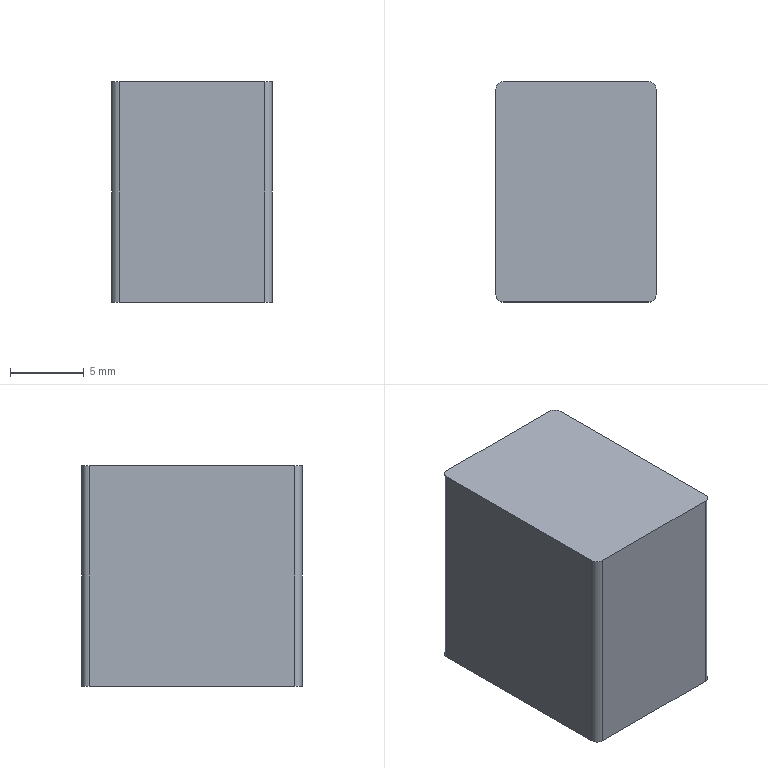Part | NX | features BREP 1 | 1 solid | 10 faces | box 10.887 x 14.955 x 15 mm | volume 2439 mm3 | plane 6 | cylinder 4 | commonest cylinder face diameters 1 x4
STEP:
#1=CARTESIAN_POINT('',(-4.944,7.478,-25.6));
#2=VERTEX_POINT('',#1);
#3=CARTESIAN_POINT('',(-5.444,6.978,-25.6));
#4=VERTEX_POINT('',#3);
#5=CARTESIAN_POINT('',(-4.944,6.978,-25.6));
#6=DIRECTION('',(0.,0.,1.));
#7=DIRECTION('',(1.,0.,0.));
#8=AXIS2_PLACEMENT_3D('',#5,#6,#7);
#9=CIRCLE('',#8,0.5);
#10=EDGE_CURVE('',#2,#4,#9,.T.);
#11=ORIENTED_EDGE('',*,*,#10,.F.);
#12=CARTESIAN_POINT('',(-4.944,7.478,-40.6));
#13=VERTEX_POINT('',#12);
#14=CARTESIAN_POINT('',(-4.944,7.478,-40.6));
#15=DIRECTION('',(0.,0.,1.));
#16=VECTOR('',#15,1000.);
#17=LINE('',#14,#16);
#18=EDGE_CURVE('',#13,#2,#17,.T.);
#19=ORIENTED_EDGE('',*,*,#18,.F.);
#20=CARTESIAN_POINT('',(-5.444,6.978,-40.6));
#21=VERTEX_POINT('',#20);
#22=CARTESIAN_POINT('',(-4.944,6.978,-40.6));
#23=DIRECTION('',(0.,0.,1.));
#24=DIRECTION('',(1.,0.,0.));
#25=AXIS2_PLACEMENT_3D('',#22,#23,#24);
#26=CIRCLE('',#25,0.5);
#27=EDGE_CURVE('',#13,#21,#26,.T.);
#28=ORIENTED_EDGE('',*,*,#27,.T.);
#29=CARTESIAN_POINT('',(-5.444,6.978,-40.6));
#30=DIRECTION('',(0.,0.,1.));
#31=VECTOR('',#30,1000.);
#32=LINE('',#29,#31);
#33=EDGE_CURVE('',#21,#4,#32,.T.);
#34=ORIENTED_EDGE('',*,*,#33,.T.);
#35=EDGE_LOOP('',(#11,#19,#28,#34));
#36=FACE_BOUND('',#35,.T.);
#37=CARTESIAN_POINT('',(-4.944,6.978,-40.6));
#38=DIRECTION('',(0.,0.,1.));
#39=DIRECTION('',(-1.,0.,0.));
#40=AXIS2_PLACEMENT_3D('',#37,#38,#39);
#41=CYLINDRICAL_SURFACE('',#40,0.5);
#42=ADVANCED_FACE('',(#36),#41,.T.);
#43=CARTESIAN_POINT('',(-5.444,-6.978,-25.6));
#44=VERTEX_POINT('',#43);
#45=CARTESIAN_POINT('',(-5.444,-6.978,-25.6));
#46=DIRECTION('',(0.,1.,0.));
#47=VECTOR('',#46,1000.);
#48=LINE('',#45,#47);
#49=EDGE_CURVE('',#44,#4,#48,.T.);
#50=ORIENTED_EDGE('',*,*,#49,.T.);
#51=ORIENTED_EDGE('',*,*,#33,.F.);
#52=CARTESIAN_POINT('',(-5.444,-6.978,-40.6));
#53=VERTEX_POINT('',#52);
#54=CARTESIAN_POINT('',(-5.444,-6.978,-40.6));
#55=DIRECTION('',(0.,1.,0.));
#56=VECTOR('',#55,1000.);
#57=LINE('',#54,#56);
#58=EDGE_CURVE('',#53,#21,#57,.T.);
#59=ORIENTED_EDGE('',*,*,#58,.F.);
#60=CARTESIAN_POINT('',(-5.444,-6.978,-40.6));
#61=DIRECTION('',(0.,0.,1.));
#62=VECTOR('',#61,1000.);
#63=LINE('',#60,#62);
#64=EDGE_CURVE('',#53,#44,#63,.T.);
#65=ORIENTED_EDGE('',*,*,#64,.T.);
#66=EDGE_LOOP('',(#50,#51,#59,#65));
#67=FACE_BOUND('',#66,.T.);
#68=CARTESIAN_POINT('',(-5.444,-6.978,-40.6));
#69=DIRECTION('',(1.,0.,0.));
#70=DIRECTION('',(0.,-1.,0.));
#71=AXIS2_PLACEMENT_3D('',#68,#69,#70);
#72=PLANE('',#71);
#73=ADVANCED_FACE('',(#67),#72,.F.);
#74=CARTESIAN_POINT('',(-4.944,-7.478,-25.6));
#75=VERTEX_POINT('',#74);
#76=CARTESIAN_POINT('',(-4.944,-6.978,-25.6));
#77=DIRECTION('',(0.,0.,1.));
#78=DIRECTION('',(1.,0.,0.));
#79=AXIS2_PLACEMENT_3D('',#76,#77,#78);
#80=CIRCLE('',#79,0.5);
#81=EDGE_CURVE('',#44,#75,#80,.T.);
#82=ORIENTED_EDGE('',*,*,#81,.F.);
#83=ORIENTED_EDGE('',*,*,#64,.F.);
#84=CARTESIAN_POINT('',(-4.944,-7.478,-40.6));
#85=VERTEX_POINT('',#84);
#86=CARTESIAN_POINT('',(-4.944,-6.978,-40.6));
#87=DIRECTION('',(0.,0.,1.));
#88=DIRECTION('',(1.,0.,0.));
#89=AXIS2_PLACEMENT_3D('',#86,#87,#88);
#90=CIRCLE('',#89,0.5);
#91=EDGE_CURVE('',#53,#85,#90,.T.);
#92=ORIENTED_EDGE('',*,*,#91,.T.);
#93=CARTESIAN_POINT('',(-4.944,-7.478,-40.6));
#94=DIRECTION('',(0.,0.,1.));
#95=VECTOR('',#94,1000.);
#96=LINE('',#93,#95);
#97=EDGE_CURVE('',#85,#75,#96,.T.);
#98=ORIENTED_EDGE('',*,*,#97,.T.);
#99=EDGE_LOOP('',(#82,#83,#92,#98));
#100=FACE_BOUND('',#99,.T.);
#101=CARTESIAN_POINT('',(-4.944,-6.978,-40.6));
#102=DIRECTION('',(0.,0.,1.));
#103=DIRECTION('',(-1.,0.,0.));
#104=AXIS2_PLACEMENT_3D('',#101,#102,#103);
#105=CYLINDRICAL_SURFACE('',#104,0.5);
#106=ADVANCED_FACE('',(#100),#105,.T.);
#107=CARTESIAN_POINT('',(4.944,-7.478,-25.6));
#108=VERTEX_POINT('',#107);
#109=CARTESIAN_POINT('',(4.944,-7.478,-25.6));
#110=DIRECTION('',(-1.,0.,0.));
#111=VECTOR('',#110,1000.);
#112=LINE('',#109,#111);
#113=EDGE_CURVE('',#108,#75,#112,.T.);
#114=ORIENTED_EDGE('',*,*,#113,.T.);
#115=ORIENTED_EDGE('',*,*,#97,.F.);
#116=CARTESIAN_POINT('',(4.944,-7.478,-40.6));
#117=VERTEX_POINT('',#116);
#118=CARTESIAN_POINT('',(4.944,-7.478,-40.6));
#119=DIRECTION('',(-1.,0.,0.));
#120=VECTOR('',#119,1000.);
#121=LINE('',#118,#120);
#122=EDGE_CURVE('',#117,#85,#121,.T.);
#123=ORIENTED_EDGE('',*,*,#122,.F.);
#124=CARTESIAN_POINT('',(4.944,-7.478,-40.6));
#125=DIRECTION('',(0.,0.,1.));
#126=VECTOR('',#125,1000.);
#127=LINE('',#124,#126);
#128=EDGE_CURVE('',#117,#108,#127,.T.);
#129=ORIENTED_EDGE('',*,*,#128,.T.);
#130=EDGE_LOOP('',(#114,#115,#123,#129));
#131=FACE_BOUND('',#130,.T.);
#132=CARTESIAN_POINT('',(4.944,-7.478,-40.6));
#133=DIRECTION('',(0.,1.,0.));
#134=DIRECTION('',(1.,0.,0.));
#135=AXIS2_PLACEMENT_3D('',#132,#133,#134);
#136=PLANE('',#135);
#137=ADVANCED_FACE('',(#131),#136,.F.);
#138=CARTESIAN_POINT('',(5.444,-6.978,-25.6));
#139=VERTEX_POINT('',#138);
#140=CARTESIAN_POINT('',(4.944,-6.978,-25.6));
#141=DIRECTION('',(0.,0.,1.));
#142=DIRECTION('',(1.,0.,0.));
#143=AXIS2_PLACEMENT_3D('',#140,#141,#142);
#144=CIRCLE('',#143,0.5);
#145=EDGE_CURVE('',#108,#139,#144,.T.);
#146=ORIENTED_EDGE('',*,*,#145,.F.);
#147=ORIENTED_EDGE('',*,*,#128,.F.);
#148=CARTESIAN_POINT('',(5.444,-6.978,-40.6));
#149=VERTEX_POINT('',#148);
#150=CARTESIAN_POINT('',(4.944,-6.978,-40.6));
#151=DIRECTION('',(0.,0.,1.));
#152=DIRECTION('',(1.,0.,0.));
#153=AXIS2_PLACEMENT_3D('',#150,#151,#152);
#154=CIRCLE('',#153,0.5);
#155=EDGE_CURVE('',#117,#149,#154,.T.);
#156=ORIENTED_EDGE('',*,*,#155,.T.);
#157=CARTESIAN_POINT('',(5.444,-6.978,-40.6));
#158=DIRECTION('',(0.,0.,1.));
#159=VECTOR('',#158,1000.);
#160=LINE('',#157,#159);
#161=EDGE_CURVE('',#149,#139,#160,.T.);
#162=ORIENTED_EDGE('',*,*,#161,.T.);
#163=EDGE_LOOP('',(#146,#147,#156,#162));
#164=FACE_BOUND('',#163,.T.);
#165=CARTESIAN_POINT('',(4.944,-6.978,-40.6));
#166=DIRECTION('',(0.,0.,1.));
#167=DIRECTION('',(-1.,0.,0.));
#168=AXIS2_PLACEMENT_3D('',#165,#166,#167);
#169=CYLINDRICAL_SURFACE('',#168,0.5);
#170=ADVANCED_FACE('',(#164),#169,.T.);
#171=CARTESIAN_POINT('',(5.444,6.978,-25.6));
#172=VERTEX_POINT('',#171);
#173=CARTESIAN_POINT('',(5.444,6.978,-25.6));
#174=DIRECTION('',(0.,-1.,0.));
#175=VECTOR('',#174,1000.);
#176=LINE('',#173,#175);
#177=EDGE_CURVE('',#172,#139,#176,.T.);
#178=ORIENTED_EDGE('',*,*,#177,.T.);
#179=ORIENTED_EDGE('',*,*,#161,.F.);
#180=CARTESIAN_POINT('',(5.444,6.978,-40.6));
#181=VERTEX_POINT('',#180);
#182=CARTESIAN_POINT('',(5.444,6.978,-40.6));
#183=DIRECTION('',(0.,-1.,0.));
#184=VECTOR('',#183,1000.);
#185=LINE('',#182,#184);
#186=EDGE_CURVE('',#181,#149,#185,.T.);
#187=ORIENTED_EDGE('',*,*,#186,.F.);
#188=CARTESIAN_POINT('',(5.444,6.978,-40.6));
#189=DIRECTION('',(0.,0.,1.));
#190=VECTOR('',#189,1000.);
#191=LINE('',#188,#190);
#192=EDGE_CURVE('',#181,#172,#191,.T.);
#193=ORIENTED_EDGE('',*,*,#192,.T.);
#194=EDGE_LOOP('',(#178,#179,#187,#193));
#195=FACE_BOUND('',#194,.T.);
#196=CARTESIAN_POINT('',(5.444,6.978,-40.6));
#197=DIRECTION('',(-1.,0.,0.));
#198=DIRECTION('',(0.,0.,-1.));
#199=AXIS2_PLACEMENT_3D('',#196,#197,#198);
#200=PLANE('',#199);
#201=ADVANCED_FACE('',(#195),#200,.F.);
#202=CARTESIAN_POINT('',(4.944,7.478,-25.6));
#203=VERTEX_POINT('',#202);
#204=CARTESIAN_POINT('',(4.944,6.978,-25.6));
#205=DIRECTION('',(0.,0.,1.));
#206=DIRECTION('',(1.,0.,0.));
#207=AXIS2_PLACEMENT_3D('',#204,#205,#206);
#208=CIRCLE('',#207,0.5);
#209=EDGE_CURVE('',#172,#203,#208,.T.);
#210=ORIENTED_EDGE('',*,*,#209,.F.);
#211=ORIENTED_EDGE('',*,*,#192,.F.);
#212=CARTESIAN_POINT('',(4.944,7.478,-40.6));
#213=VERTEX_POINT('',#212);
#214=CARTESIAN_POINT('',(4.944,6.978,-40.6));
#215=DIRECTION('',(0.,0.,1.));
#216=DIRECTION('',(1.,0.,0.));
#217=AXIS2_PLACEMENT_3D('',#214,#215,#216);
#218=CIRCLE('',#217,0.5);
#219=EDGE_CURVE('',#181,#213,#218,.T.);
#220=ORIENTED_EDGE('',*,*,#219,.T.);
#221=CARTESIAN_POINT('',(4.944,7.478,-40.6));
#222=DIRECTION('',(0.,0.,1.));
#223=VECTOR('',#222,1000.);
#224=LINE('',#221,#223);
#225=EDGE_CURVE('',#213,#203,#224,.T.);
#226=ORIENTED_EDGE('',*,*,#225,.T.);
#227=EDGE_LOOP('',(#210,#211,#220,#226));
#228=FACE_BOUND('',#227,.T.);
#229=CARTESIAN_POINT('',(4.944,6.978,-40.6));
#230=DIRECTION('',(0.,0.,1.));
#231=DIRECTION('',(-1.,0.,0.));
#232=AXIS2_PLACEMENT_3D('',#229,#230,#231);
#233=CYLINDRICAL_SURFACE('',#232,0.5);
#234=ADVANCED_FACE('',(#228),#233,.T.);
#235=CARTESIAN_POINT('',(-4.944,7.478,-25.6));
#236=DIRECTION('',(1.,0.,0.));
#237=VECTOR('',#236,1000.);
#238=LINE('',#235,#237);
#239=EDGE_CURVE('',#2,#203,#238,.T.);
#240=ORIENTED_EDGE('',*,*,#239,.T.);
#241=ORIENTED_EDGE('',*,*,#225,.F.);
#242=CARTESIAN_POINT('',(-4.944,7.478,-40.6));
#243=DIRECTION('',(1.,0.,0.));
#244=VECTOR('',#243,1000.);
#245=LINE('',#242,#244);
#246=EDGE_CURVE('',#13,#213,#245,.T.);
#247=ORIENTED_EDGE('',*,*,#246,.F.);
#248=ORIENTED_EDGE('',*,*,#18,.T.);
#249=EDGE_LOOP('',(#240,#241,#247,#248));
#250=FACE_BOUND('',#249,.T.);
#251=CARTESIAN_POINT('',(-4.944,7.478,-40.6));
#252=DIRECTION('',(0.,-1.,0.));
#253=DIRECTION('',(0.,0.,1.));
#254=AXIS2_PLACEMENT_3D('',#251,#252,#253);
#255=PLANE('',#254);
#256=ADVANCED_FACE('',(#250),#255,.F.);
#257=ORIENTED_EDGE('',*,*,#27,.F.);
#258=ORIENTED_EDGE('',*,*,#246,.T.);
#259=ORIENTED_EDGE('',*,*,#219,.F.);
#260=ORIENTED_EDGE('',*,*,#186,.T.);
#261=ORIENTED_EDGE('',*,*,#155,.F.);
#262=ORIENTED_EDGE('',*,*,#122,.T.);
#263=ORIENTED_EDGE('',*,*,#91,.F.);
#264=ORIENTED_EDGE('',*,*,#58,.T.);
#265=EDGE_LOOP('',(#257,#258,#259,#260,#261,#262,#263,#264));
#266=FACE_BOUND('',#265,.T.);
#267=CARTESIAN_POINT('',(-4.944,6.978,-40.6));
#268=DIRECTION('',(0.,0.,1.));
#269=DIRECTION('',(-1.,0.,0.));
#270=AXIS2_PLACEMENT_3D('',#267,#268,#269);
#271=PLANE('',#270);
#272=ADVANCED_FACE('',(#266),#271,.F.);
#273=ORIENTED_EDGE('',*,*,#10,.T.);
#274=ORIENTED_EDGE('',*,*,#49,.F.);
#275=ORIENTED_EDGE('',*,*,#81,.T.);
#276=ORIENTED_EDGE('',*,*,#113,.F.);
#277=ORIENTED_EDGE('',*,*,#145,.T.);
#278=ORIENTED_EDGE('',*,*,#177,.F.);
#279=ORIENTED_EDGE('',*,*,#209,.T.);
#280=ORIENTED_EDGE('',*,*,#239,.F.);
#281=EDGE_LOOP('',(#273,#274,#275,#276,#277,#278,#279,#280));
#282=FACE_BOUND('',#281,.T.);
#283=CARTESIAN_POINT('',(-4.944,6.978,-25.6));
#284=DIRECTION('',(0.,0.,1.));
#285=DIRECTION('',(-1.,0.,0.));
#286=AXIS2_PLACEMENT_3D('',#283,#284,#285);
#287=PLANE('',#286);
#288=ADVANCED_FACE('',(#282),#287,.T.);
#289=CLOSED_SHELL('',(#42,#73,#106,#137,#170,#201,#234,#256,#272,#288));
#290=MANIFOLD_SOLID_BREP('',#289);
#291=(LENGTH_UNIT()NAMED_UNIT(*)SI_UNIT(.MILLI.,.METRE.));
#292=UNCERTAINTY_MEASURE_WITH_UNIT(LENGTH_MEASURE(0.00001),#291,'','');
#293=(NAMED_UNIT(*)PLANE_ANGLE_UNIT()SI_UNIT($,.RADIAN.));
#294=(NAMED_UNIT(*)SI_UNIT($,.STERADIAN.)SOLID_ANGLE_UNIT());
#295=(GEOMETRIC_REPRESENTATION_CONTEXT(3)GLOBAL_UNCERTAINTY_ASSIGNED_CONTEXT((#292))GLOBAL_UNIT_ASSIGNED_CONTEXT((#291,#293,#294))REPRESENTATION_CONTEXT('',''));
#296=ADVANCED_BREP_SHAPE_REPRESENTATION('',(#290),#295);